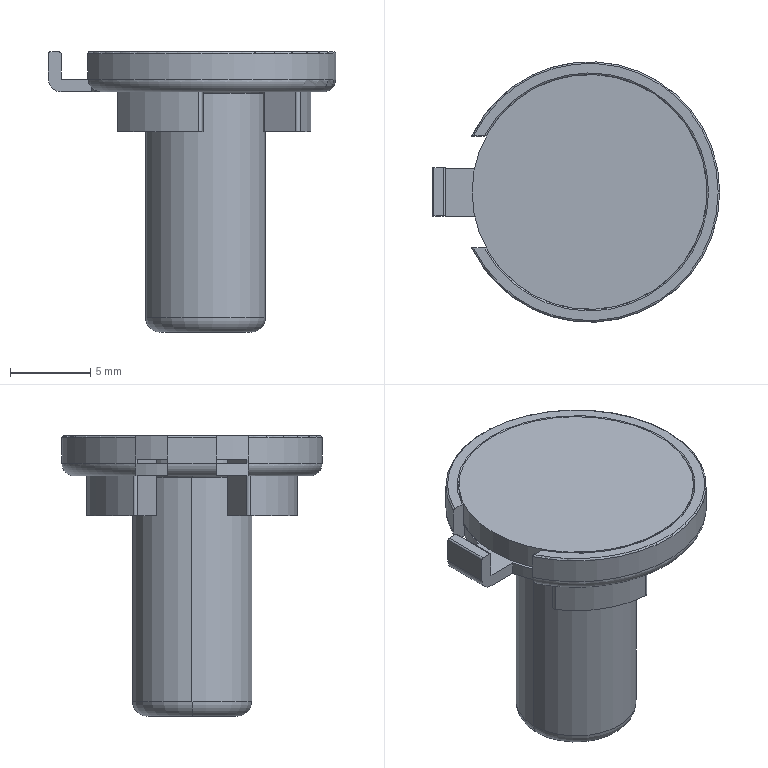NC program | NX | posted with a generic post | part box 17.958 x 16.273 x 17.5 mm
Lines 901 to 1957 of 9718:
(ZLEVEL_PROFILE_COPY_1 , TOOL : D2)
N1782 T02 M6
N1784 G54
N1786 G17 G0 G90 X-10.478 Y2.889 S6500 M3
N1788 G43 Z10.5 H2
N1790 Z-0.04
N1792 G94 G1 X-10.31 Y2.598 F1250.
N1794 G3 X-10.137 Y2.498 R0.2
N1796 G1 X-9.965
N1798 X-9.951 Y2.5
N1800 X-8.536
N1802 G3 X-8.362 Y2.6 R0.2
N1804 G1 X-9.107 Y2.9
N1806 G0 X-10.478 Y2.889 Z-0.079
N1808 G1 X-10.31 Y2.598
N1810 G3 X-10.137 Y2.498 R0.2
N1812 G1 X-9.965
N1814 X-9.951 Y2.5
N1816 X-8.536
N1818 G3 X-8.362 Y2.6 R0.2
N1820 G1 X-9.108 Y2.9
N1822 G0 X-10.478 Y2.889 Z-0.119
N1824 G1 X-10.31 Y2.598
N1826 G3 X-10.137 Y2.498 R0.2
N1828 G1 X-10.04
N1830 X-9.976 Y2.488
N1832 X-9.965 Y2.498
N1834 X-9.801 Y2.5
N1836 X-8.536
N1838 G3 X-8.362 Y2.6 R0.2
N1840 G1 X-9.108 Y2.9
N1842 G0 X-10.479 Y2.889 Z-0.159
N1844 G1 X-10.31 Y2.598
N1846 G3 X-10.137 Y2.498 R0.2
N1848 G1 X-10.04
N1850 X-9.976 Y2.488
N1852 X-9.965 Y2.498
N1854 X-9.801 Y2.5
N1856 X-8.536
N1858 G3 X-8.362 Y2.6 R0.2
N1860 G1 X-9.108 Y2.9
N1862 G0 X-10.479 Y2.889 Z-0.198
N1864 G1 X-10.311 Y2.598
N1866 G3 X-10.137 Y2.498 R0.2
N1868 G1 X-10.04
N1870 X-9.976 Y2.488
N1872 X-9.965 Y2.498
N1874 X-9.801 Y2.5
N1876 X-8.536
N1878 G3 X-8.362 Y2.6 R0.2
N1880 G1 X-9.108 Y2.9
N1882 G0 X-10.479 Y2.889 Z-0.238
N1884 G1 X-10.311 Y2.598
N1886 G3 X-10.138 Y2.498 R0.2
N1888 G1 X-10.04
N1890 X-9.976 Y2.488
N1892 X-9.965 Y2.498
N1894 X-9.801 Y2.5
N1896 X-8.536
N1898 G3 X-8.362 Y2.6 R0.2
N1900 G1 X-9.108 Y2.9
N1902 G0 X-10.479 Y2.889 Z-0.278
N1904 G1 X-10.311 Y2.598
N1906 G3 X-10.138 Y2.498 R0.2
N1908 G1 X-10.04
N1910 X-9.976 Y2.488
N1912 X-9.965 Y2.498
N1914 X-9.801 Y2.5
N1916 X-8.536
N1918 G3 X-8.362 Y2.6 R0.2
N1920 G1 X-9.108 Y2.9
N1922 G0 X-10.479 Y2.889 Z-0.317
N1924 G1 X-10.311 Y2.598
N1926 G3 X-10.138 Y2.498 R0.2
N1928 G1 X-10.04
N1930 X-9.976 Y2.488
N1932 X-9.965 Y2.498
N1934 X-9.801 Y2.5
N1936 X-8.536
N1938 G3 X-8.362 Y2.6 R0.2
N1940 G1 X-9.108 Y2.9
N1942 G0 X-10.479 Y2.889 Z-0.357
N1944 G1 X-10.311 Y2.598
N1946 G3 X-10.138 Y2.498 R0.2
N1948 G1 X-10.04
N1950 X-9.976 Y2.488
N1952 X-9.965 Y2.498
N1954 X-9.801 Y2.5
N1956 X-8.536
N1958 G3 X-8.362 Y2.6 R0.2
N1960 G1 X-9.108 Y2.9
N1962 G0 X-10.479 Y2.889 Z-0.397
N1964 G1 X-10.311 Y2.598
N1966 G3 X-10.138 Y2.498 R0.2
N1968 G1 X-10.04
N1970 X-9.976 Y2.488
N1972 X-9.965 Y2.498
N1974 X-9.801 Y2.5
N1976 X-8.536
N1978 G3 X-8.362 Y2.6 R0.2
N1980 G1 X-9.108 Y2.9
N1982 G0 X-10.479 Y2.889 Z-0.437
N1984 G1 X-10.311 Y2.598
N1986 G3 X-10.138 Y2.498 R0.2
N1988 G1 X-10.04
N1990 X-9.976 Y2.488
N1992 X-9.965 Y2.498
N1994 X-9.801 Y2.5
N1996 X-8.536
N1998 G3 X-8.362 Y2.6 R0.2
N2000 G1 X-9.108 Y2.9
N2002 G0 X-10.48 Y2.889 Z-0.476
N2004 G1 X-10.312 Y2.598
N2006 G3 X-10.138 Y2.498 R0.2
N2008 G1 X-10.04
N2010 X-9.976 Y2.488
N2012 X-9.965 Y2.498
N2014 X-9.801 Y2.5
N2016 X-8.536
N2018 G3 X-8.362 Y2.6 R0.2
N2020 G1 X-9.108 Y2.9
N2022 G0 X-10.48 Y2.889 Z-0.516
N2024 G1 X-10.312 Y2.598
N2026 G3 X-10.139 Y2.498 R0.2
N2028 G1 X-10.04
N2030 X-9.976 Y2.488
N2032 X-9.965 Y2.498
N2034 X-9.801 Y2.5
N2036 X-8.536
N2038 G3 X-8.362 Y2.6 R0.2
N2040 G1 X-9.108 Y2.9
N2042 G0 X-10.48 Y2.889 Z-0.556
N2044 G1 X-10.312 Y2.598
N2046 G3 X-10.139 Y2.498 R0.2
N2048 G1 X-10.04
N2050 X-9.976 Y2.488
N2052 X-9.965 Y2.498
N2054 X-9.801 Y2.5
N2056 X-8.536
N2058 G3 X-8.362 Y2.6 R0.2
N2060 G1 X-9.108 Y2.9
N2062 G0 X-10.48 Y2.889 Z-0.595
N2064 G1 X-10.312 Y2.598
N2066 G3 X-10.139 Y2.498 R0.2
N2068 G1 X-10.04
N2070 X-9.976 Y2.488
N2072 X-9.965 Y2.498
N2074 X-9.801 Y2.5
N2076 X-8.536
N2078 G3 X-8.362 Y2.6 R0.2
N2080 G1 X-9.108 Y2.9
N2082 G0 X-10.48 Y2.889 Z-0.635
N2084 G1 X-10.312 Y2.598
N2086 G3 X-10.139 Y2.498 R0.2
N2088 G1 X-10.04
N2090 X-9.976 Y2.488
N2092 X-9.965 Y2.498
N2094 X-9.801 Y2.5
N2096 X-8.536
N2098 G3 X-8.362 Y2.6 R0.2
N2100 G1 X-9.108 Y2.9
N2102 G0 X-10.48 Y2.889 Z-0.675
N2104 G1 X-10.312 Y2.598
N2106 G3 X-10.139 Y2.498 R0.2
N2108 G1 X-10.04
N2110 X-9.976 Y2.488
N2112 X-9.965 Y2.498
N2114 X-9.801 Y2.5
N2116 X-8.536
N2118 G3 X-8.362 Y2.6 R0.2
N2120 G1 X-9.108 Y2.9
N2122 G0 X-10.48 Y2.889 Z-0.714
N2124 G1 X-10.313 Y2.599
N2126 G3 X-10.139 Y2.498 R0.2
N2128 G1 X-10.04
N2130 X-9.976 Y2.488
N2132 X-9.965 Y2.498
N2134 X-9.801 Y2.5
N2136 X-8.536
N2138 G3 X-8.362 Y2.6 R0.2
N2140 G1 X-9.108 Y2.9
N2142 G0 X-10.48 Y2.889 Z-0.754
N2144 G1 X-10.313 Y2.599
N2146 G3 X-10.14 Y2.498 R0.2
N2148 G1 X-10.04
N2150 X-9.976 Y2.488
N2152 X-9.965 Y2.498
N2154 X-9.801 Y2.5
N2156 X-8.536
N2158 G3 X-8.362 Y2.6 R0.2
N2160 G1 X-9.108 Y2.9
N2162 G0 X-10.48 Y2.889 Z-0.794
N2164 G1 X-10.313 Y2.599
N2166 G3 X-10.14 Y2.499 R0.2
N2168 G1 X-10.04 Y2.498
N2170 X-9.976 Y2.488
N2172 X-9.965 Y2.498
N2174 X-9.801 Y2.5
N2176 X-8.536
N2178 G3 X-8.362 Y2.6 R0.2
N2180 G1 X-9.108 Y2.9
N2182 G0 X-10.481 Y2.889 Z-0.833
N2184 G1 X-10.313 Y2.599
N2186 G3 X-10.14 Y2.499 R0.2
N2188 G1 X-10.04 Y2.498
N2190 X-9.976 Y2.488
N2192 X-9.965 Y2.498
N2194 X-9.801 Y2.5
N2196 X-8.536
N2198 G3 X-8.362 Y2.6 R0.2
N2200 G1 X-9.108 Y2.9
N2202 G0 X-10.481 Y2.89 Z-0.873
N2204 G1 X-10.313 Y2.599
N2206 G3 X-10.14 Y2.499 R0.2
N2208 G1 X-10.04 Y2.498
N2210 X-9.976 Y2.488
N2212 X-9.965 Y2.498
N2214 X-9.801 Y2.5
N2216 X-8.536
N2218 G3 X-8.362 Y2.6 R0.2
N2220 G1 X-9.108 Y2.9
N2222 G0 X-10.481 Y2.89 Z-0.913
N2224 G1 X-10.313 Y2.599
N2226 G3 X-10.14 Y2.499 R0.2
N2228 G1 X-10.04
N2230 X-9.976 Y2.488
N2232 X-9.965 Y2.499
N2234 X-9.801 Y2.5
N2236 X-8.536
N2238 G3 X-8.362 Y2.6 R0.2
N2240 G1 X-9.108 Y2.9
N2242 G0 X-10.481 Y2.89 Z-0.952
N2244 G1 X-10.313 Y2.599
N2246 G3 X-10.14 Y2.499 R0.2
N2248 G1 X-10.04
N2250 X-9.976 Y2.488
N2252 X-9.965 Y2.499
N2254 X-9.801 Y2.5
N2256 X-8.536
N2258 G3 X-8.362 Y2.6 R0.2
N2260 G1 X-9.108 Y2.9
N2262 G0 X-10.481 Y2.89 Z-0.992
N2264 G1 X-10.314 Y2.599
N2266 G3 X-10.14 Y2.499 R0.2
N2268 G1 X-10.04
N2270 X-9.976 Y2.488
N2272 X-9.965 Y2.499
N2274 X-9.801 Y2.5
N2276 X-8.536
N2278 G3 X-8.362 Y2.6 R0.2
N2280 G1 X-9.108 Y2.9
N2282 G0 X-10.481 Y2.89 Z-1.032
N2284 G1 X-10.314 Y2.599
N2286 G3 X-10.141 Y2.499 R0.2
N2288 G1 X-10.04
N2290 X-9.976 Y2.488
N2292 X-9.965 Y2.499
N2294 X-9.801 Y2.5
N2296 X-8.536
N2298 G3 X-8.362 Y2.6 R0.2
N2300 G1 X-9.108 Y2.9
N2302 G0 X-10.481 Y2.89 Z-1.071
N2304 G1 X-10.314 Y2.599
N2306 G3 X-10.141 Y2.499 R0.2
N2308 G1 X-10.04
N2310 X-9.976 Y2.488
N2312 X-9.965 Y2.499
N2314 X-9.801 Y2.5
N2316 X-8.536
N2318 G3 X-8.362 Y2.6 R0.2
N2320 G1 X-9.108 Y2.9
N2322 G0 X-10.481 Y2.89 Z-1.111
N2324 G1 X-10.314 Y2.599
N2326 G3 X-10.141 Y2.499 R0.2
N2328 G1 X-10.04
N2330 X-9.976 Y2.488
N2332 X-9.965 Y2.499
N2334 X-9.801 Y2.5
N2336 X-8.536
N2338 G3 X-8.362 Y2.6 R0.2
N2340 G1 X-9.108 Y2.9
N2342 G0 X-10.481 Y2.89 Z-1.151
N2344 G1 X-10.314 Y2.599
N2346 G3 X-10.141 Y2.499 R0.2
N2348 G1 X-10.04
N2350 X-9.976 Y2.488
N2352 X-9.965 Y2.499
N2354 X-9.801 Y2.5
N2356 X-8.536
N2358 G3 X-8.362 Y2.6 R0.2
N2360 G1 X-9.108 Y2.9
N2362 G0 X-10.482 Y2.89 Z-1.19
N2364 G1 X-10.314 Y2.599
N2366 G3 X-10.141 Y2.499 R0.2
N2368 G1 X-10.04
N2370 X-9.976 Y2.488
N2372 X-9.965 Y2.499
N2374 X-9.801 Y2.5
N2376 X-8.536
N2378 G3 X-8.362 Y2.6 R0.2
N2380 G1 X-9.109 Y2.9
N2382 G0 X-10.482 Y2.89 Z-1.23
N2384 G1 X-10.314 Y2.599
N2386 G3 X-10.141 Y2.499 R0.2
N2388 G1 X-10.04
N2390 X-9.976 Y2.488
N2392 X-9.965 Y2.499
N2394 X-9.801 Y2.5
N2396 X-7.882
N2398 G0 X-10.482 Y2.89 Z-1.27
N2400 G1 X-10.315 Y2.599
N2402 G3 X-10.142 Y2.499 R0.2
N2404 G1 X-10.04
N2406 X-9.976 Y2.488
N2408 X-9.965 Y2.499
N2410 X-9.801 Y2.5
N2412 X-7.882
N2414 G0 X-10.482 Y2.89 Z-1.31
N2416 G1 X-10.315 Y2.599
N2418 G3 X-10.142 Y2.499 R0.2
N2420 G1 X-10.04
N2422 X-9.976 Y2.488
N2424 X-9.965 Y2.499
N2426 X-9.801 Y2.5
N2428 X-7.883
N2430 G0 X-10.482 Y2.89 Z-1.349
N2432 G1 X-10.315 Y2.599
N2434 G3 X-10.142 Y2.499 R0.2
N2436 G1 X-10.04
N2438 X-9.976 Y2.488
N2440 X-9.965 Y2.499
N2442 X-9.801 Y2.5
N2444 X-7.883
N2446 G0 X-10.482 Y2.89 Z-1.389
N2448 G1 X-10.315 Y2.599
N2450 G3 X-10.142 Y2.499 R0.2
N2452 G1 X-10.04
N2454 X-9.976 Y2.488
N2456 X-9.965 Y2.499
N2458 X-9.801 Y2.5
N2460 X-7.883
N2462 G0 X-10.482 Y2.89 Z-1.429
N2464 G1 X-10.315 Y2.6
N2466 G3 X-10.142 Y2.499 R0.2
N2468 G1 X-10.04
N2470 X-9.976 Y2.488
N2472 X-9.965 Y2.499
N2474 X-9.801 Y2.5
N2476 X-7.884
N2478 G0 X-10.482 Y2.89 Z-1.468
N2480 G1 X-10.315 Y2.6
N2482 G3 X-10.142 Y2.499 R0.2
N2484 G1 X-10.04
N2486 X-9.976 Y2.488
N2488 X-9.965 Y2.499
N2490 X-9.801 Y2.5
N2492 X-7.884
N2494 G0 X-10.482 Y2.89 Z-1.508
N2496 G1 X-10.316 Y2.6
N2498 G3 X-10.142 Y2.499 R0.2
N2500 G1 X-10.04
N2502 X-9.976 Y2.488
N2504 X-9.965 Y2.499
N2506 X-9.801 Y2.5
N2508 X-7.884
N2510 G0 X-10.483 Y2.89 Z-1.548
N2512 G1 X-10.316 Y2.6
N2514 G3 X-10.143 Y2.499 R0.2
N2516 G1 X-10.04
N2518 X-9.976 Y2.488
N2520 X-9.965 Y2.499
N2522 X-9.801 Y2.5
N2524 X-7.885
N2526 G0 X-10.483 Y2.89 Z-1.587
N2528 G1 X-10.316 Y2.6
N2530 G3 X-10.143 Y2.499 R0.2
N2532 G1 X-10.04
N2534 X-9.976 Y2.488
N2536 X-9.965 Y2.499
N2538 X-9.801 Y2.5
N2540 X-7.885
N2542 G0 X-10.483 Y2.89 Z-1.627
N2544 G1 X-10.316 Y2.6
N2546 G3 X-10.143 Y2.499 R0.2
N2548 G1 X-10.04
N2550 X-9.976 Y2.488
N2552 X-9.965 Y2.499
N2554 X-9.801 Y2.5
N2556 X-7.885
N2558 G0 X-10.483 Y2.89 Z-1.667
N2560 G1 X-10.316 Y2.6
N2562 G3 X-10.143 Y2.499 R0.2
N2564 G1 X-10.04
N2566 X-9.976 Y2.488
N2568 X-9.965 Y2.499
N2570 X-9.801 Y2.5
N2572 X-7.886
N2574 G0 X-10.483 Y2.89 Z-1.706
N2576 G1 X-10.316 Y2.6
N2578 G3 X-10.143 Y2.5 R0.2
N2580 G1 X-10.04 Y2.499
N2582 X-9.976 Y2.488
N2584 X-9.965 Y2.499
N2586 X-9.801 Y2.5
N2588 X-7.886
N2590 G0 X-10.483 Y2.89 Z-1.746
N2592 G1 X-10.316 Y2.6
N2594 G3 X-10.143 Y2.5 R0.2
N2596 G1 X-10.04 Y2.499
N2598 X-9.976 Y2.488
N2600 X-9.965 Y2.499
N2602 X-9.801 Y2.5
N2604 X-7.886
N2606 G0 X-10.483 Y2.89 Z-1.786
N2608 G1 X-10.317 Y2.6
N2610 G3 X-10.144 Y2.5 R0.2
N2612 G1 X-10.04 Y2.499
N2614 X-9.976 Y2.488
N2616 X-9.965 Y2.499
N2618 X-9.801 Y2.5
N2620 X-7.886
N2622 G0 X-10.484 Y2.89 Z-1.825
N2624 G1 X-10.317 Y2.6
N2626 G3 X-10.144 Y2.5 R0.2
N2628 G1 X-10.04 Y2.499
N2630 X-9.976 Y2.488
N2632 X-9.965 Y2.499
N2634 X-9.801 Y2.5
N2636 X-7.886
N2638 G0 X-10.484 Y2.89 Z-1.865
N2640 G1 X-10.317 Y2.6
N2642 G3 X-10.144 Y2.5 R0.2
N2644 G1 X-10.04 Y2.499
N2646 X-9.976 Y2.488
N2648 X-9.965 Y2.499
N2650 X-9.801 Y2.5
N2652 X-7.886
N2654 G0 X-10.484 Y2.89 Z-1.905
N2656 G1 X-10.317 Y2.6
N2658 G3 X-10.144 Y2.5 R0.2
N2660 G1 X-10.04 Y2.499
N2662 X-9.976 Y2.488
N2664 X-9.965 Y2.499
N2666 X-9.795 Y2.5
N2668 X-7.886
N2670 G0 X-10.484 Y2.89 Z-1.944
N2672 G1 X-10.317 Y2.6
N2674 G3 X-10.144 Y2.5 R0.2
N2676 G1 X-10.04 Y2.499
N2678 X-9.976 Y2.488
N2680 X-9.965 Y2.499
N2682 X-9.785 Y2.5
N2684 X-7.886
N2686 G0 X-10.484 Y2.89 Z-1.984
N2688 G1 X-10.317 Y2.6
N2690 G3 X-10.144 Y2.5 R0.2
N2692 G1 X-10.04
N2694 X-9.976 Y2.488
N2696 X-9.965 Y2.499
N2698 X-9.785 Y2.5
N2700 X-7.886
N2702 G0 X-10.485 Y2.89 Z-2.024
N2704 G1 X-10.318 Y2.6
N2706 G3 X-10.145 Y2.5 R0.2
N2708 G1 X-10.04
N2710 X-9.976 Y2.488
N2712 X-9.965 Y2.5
N2714 X-9.785
N2716 X-7.886
N2718 G0 X-10.485 Y2.89 Z-2.063
N2720 G1 X-10.318 Y2.6
N2722 G3 X-10.145 Y2.5 R0.2
N2724 G1 X-10.04
N2726 X-9.976 Y2.488
N2728 X-9.965 Y2.5
N2730 X-9.785
N2732 X-7.886
N2734 G0 X-10.485 Y2.89 Z-2.103
N2736 G1 X-10.318 Y2.6
N2738 G3 X-10.145 Y2.5 R0.2
N2740 G1 X-10.04
N2742 X-9.976 Y2.488
N2744 X-9.965 Y2.5
N2746 X-9.785
N2748 X-7.886
N2750 G0 X-10.485 Y2.89 Z-2.143
N2752 G1 X-10.318 Y2.6
N2754 G3 X-10.145 Y2.5 R0.2
N2756 G1 X-10.04
N2758 X-9.976 Y2.488
N2760 X-9.965 Y2.5
N2762 X-9.785
N2764 X-7.886
N2766 G0 X-10.485 Y2.89 Z-2.183
N2768 G1 X-10.318 Y2.6
N2770 G3 X-10.145 Y2.5 R0.2
N2772 G1 X-10.04
N2774 X-9.976 Y2.488
N2776 X-9.965 Y2.5
N2778 X-9.785
N2780 X-7.886
N2782 G0 X-10.486 Y2.89 Z-2.222
N2784 G1 X-10.318 Y2.6
N2786 G3 X-10.145 Y2.5 R0.2
N2788 G1 X-10.04
N2790 X-9.976 Y2.488
N2792 X-9.965 Y2.5
N2794 X-9.785
N2796 X-7.886
N2798 G0 X-10.486 Y2.89 Z-2.262
N2800 G1 X-10.319 Y2.6
N2802 G3 X-10.145 Y2.5 R0.2
N2804 G1 X-10.04
N2806 X-9.976 Y2.488
N2808 X-9.965 Y2.5
N2810 X-9.785
N2812 X-7.886
N2814 G0 X-10.486 Y2.89 Z-2.302
N2816 G1 X-10.319 Y2.6
N2818 G3 X-10.146 Y2.5 R0.2
N2820 G1 X-10.04
N2822 X-9.976 Y2.488
N2824 X-9.965 Y2.5
N2826 X-9.785
N2828 X-7.886
N2830 G0 X-10.486 Y2.89 Z-2.341
N2832 G1 X-10.319 Y2.6
N2834 G3 X-10.146 Y2.5 R0.2
N2836 G1 X-10.04
N2838 X-9.976 Y2.488
N2840 X-9.965 Y2.5
N2842 X-9.785
N2844 X-7.886
N2846 G0 X-10.486 Y2.89 Z-2.381
N2848 G1 X-10.319 Y2.6
N2850 G3 X-10.146 Y2.5 R0.2
N2852 G1 X-10.04
N2854 X-9.976 Y2.488
N2856 X-9.965 Y2.5
N2858 X-9.785
N2860 X-7.886
N2862 G0 X-10.487 Y2.89 Z-2.421
N2864 G1 X-10.319 Y2.6
N2866 G3 X-10.146 Y2.5 R0.2
N2868 G1 X-10.04
N2870 X-9.976 Y2.488
N2872 X-9.965 Y2.5
N2874 X-9.785
N2876 X-7.886
N2878 G0 X-10.487 Y2.89 Z-2.46
N2880 G1 X-10.319 Y2.6
N2882 G3 X-10.146 Y2.5 R0.2
N2884 G1 X-10.04
N2886 X-9.976 Y2.488
N2888 X-9.965 Y2.5
N2890 X-9.785
N2892 X-7.886
N2894 G0 X-10.486 Y2.89 Z-2.5
N2896 G1 X-10.319 Y2.6
N2898 G3 X-10.146 Y2.5 R0.2
N2900 G1 X-10.027 Y2.499
N2902 X-9.976 Y2.488
N2904 X-9.965 Y2.5
N2906 X-9.785
N2908 X-7.886
N2910 G0 Z10.5
N2912 X-9.108 Y-2.9
N2914 Z-0.04
N2916 G1 X-8.356 Y-2.6
N2918 G3 X-8.529 Y-2.5 R0.2
N2920 G1 X-9.817
N2922 X-9.829 Y-2.497
N2924 X-10.135
N2926 G3 X-10.308 Y-2.597 R0.2
N2928 G1 X-10.477 Y-2.888
N2930 G0 X-9.109 Y-2.9 Z-0.079
N2932 G1 X-8.356 Y-2.6
N2934 G3 X-8.529 Y-2.5 R0.2
N2936 G1 X-9.82
N2938 X-10.135 Y-2.498
N2940 G3 X-10.309 Y-2.597 R0.2
N2942 G1 X-10.48 Y-2.888
N2944 G0 X-9.108 Y-2.9 Z-0.119
N2946 G1 X-8.356 Y-2.6
N2948 G3 X-8.529 Y-2.5 R0.2
N2950 G1 X-9.821
N2952 X-10.135 Y-2.498
N2954 G3 X-10.309 Y-2.597 R0.2
N2956 G1 X-10.48 Y-2.888
N2958 G0 X-9.108 Y-2.9 Z-0.159
N2960 G1 X-8.356 Y-2.6
N2962 G3 X-8.529 Y-2.5 R0.2
N2964 G1 X-9.821
N2966 X-10.135 Y-2.498
N2968 G3 X-10.309 Y-2.597 R0.2
N2970 G1 X-10.48 Y-2.888
N2972 G0 X-9.108 Y-2.9 Z-0.198
N2974 G1 X-8.356 Y-2.6
N2976 G3 X-8.529 Y-2.5 R0.2
N2978 G1 X-9.821
N2980 X-10.136 Y-2.498
N2982 G3 X-10.309 Y-2.597 R0.2
N2984 G1 X-10.48 Y-2.888
N2986 G0 X-9.108 Y-2.9 Z-0.238
N2988 G1 X-8.356 Y-2.6
N2990 G3 X-8.529 Y-2.5 R0.2
N2992 G1 X-9.821
N2994 X-10.136 Y-2.498
N2996 G3 X-10.309 Y-2.597 R0.2
N2998 G1 X-10.48 Y-2.888
N3000 G0 X-9.108 Y-2.9 Z-0.278
N3002 G1 X-8.356 Y-2.6
N3004 G3 X-8.529 Y-2.5 R0.2
N3006 G1 X-9.821
N3008 X-10.136 Y-2.498
N3010 G3 X-10.31 Y-2.597 R0.2
N3012 G1 X-10.48 Y-2.888
N3014 G0 X-9.109 Y-2.9 Z-0.317
N3016 G1 X-8.356 Y-2.6
N3018 G3 X-8.529 Y-2.5 R0.2
N3020 G1 X-9.821
N3022 X-10.136 Y-2.498
N3024 G3 X-10.31 Y-2.597 R0.2
N3026 G1 X-10.48 Y-2.888
N3028 G0 X-9.109 Y-2.9 Z-0.357
N3030 G1 X-8.356 Y-2.6
N3032 G3 X-8.529 Y-2.5 R0.2
N3034 G1 X-9.821
N3036 X-10.136 Y-2.498
N3038 G3 X-10.31 Y-2.597 R0.2
N3040 G1 X-10.48 Y-2.888
N3042 G0 X-9.109 Y-2.9 Z-0.397
N3044 G1 X-8.356 Y-2.6
N3046 G3 X-8.529 Y-2.5 R0.2
N3048 G1 X-9.821
N3050 X-10.136 Y-2.498
N3052 G3 X-10.31 Y-2.597 R0.2
N3054 G1 X-10.48 Y-2.888
N3056 G0 X-9.109 Y-2.9 Z-0.437
N3058 G1 X-8.356 Y-2.6
N3060 G3 X-8.529 Y-2.5 R0.2
N3062 G1 X-9.821
N3064 X-10.136 Y-2.498
N3066 G3 X-10.31 Y-2.597 R0.2
N3068 G1 X-10.48 Y-2.888
N3070 G0 X-9.109 Y-2.9 Z-0.476
N3072 G1 X-8.356 Y-2.6
N3074 G3 X-8.529 Y-2.5 R0.2
N3076 G1 X-9.821
N3078 X-10.136 Y-2.498
N3080 G3 X-10.31 Y-2.597 R0.2
N3082 G1 X-10.48 Y-2.888
N3084 G0 X-9.109 Y-2.9 Z-0.516
N3086 G1 X-8.356 Y-2.6
N3088 G3 X-8.529 Y-2.5 R0.2
N3090 G1 X-9.821
N3092 X-10.136 Y-2.498
N3094 G3 X-10.31 Y-2.597 R0.2
N3096 G1 X-10.48 Y-2.888
N3098 G0 X-9.109 Y-2.9 Z-0.556
N3100 G1 X-8.356 Y-2.6
N3102 G3 X-8.529 Y-2.5 R0.2
N3104 G1 X-9.821
N3106 X-10.136 Y-2.498
N3108 G3 X-10.31 Y-2.597 R0.2
N3110 G1 X-10.48 Y-2.888
N3112 G0 X-9.109 Y-2.9 Z-0.595
N3114 G1 X-8.356 Y-2.6
N3116 G3 X-8.529 Y-2.5 R0.2
N3118 G1 X-9.821
N3120 X-10.136 Y-2.498
N3122 G3 X-10.31 Y-2.597 R0.2
N3124 G1 X-10.48 Y-2.888
N3126 G0 X-9.109 Y-2.9 Z-0.635
N3128 G1 X-8.356 Y-2.6
N3130 G3 X-8.529 Y-2.5 R0.2
N3132 G1 X-9.821
N3134 X-10.136 Y-2.498
N3136 G3 X-10.31 Y-2.597 R0.2
N3138 G1 X-10.481 Y-2.888
N3140 G0 X-9.109 Y-2.9 Z-0.675
N3142 G1 X-8.356 Y-2.6
N3144 G3 X-8.529 Y-2.5 R0.2
N3146 G1 X-9.821
N3148 X-10.137 Y-2.498
N3150 G3 X-10.31 Y-2.597 R0.2
N3152 G1 X-10.481 Y-2.888
N3154 G0 X-9.109 Y-2.9 Z-0.714
N3156 G1 X-8.356 Y-2.6
N3158 G3 X-8.529 Y-2.5 R0.2
N3160 G1 X-9.821
N3162 X-10.137 Y-2.498
N3164 G3 X-10.31 Y-2.597 R0.2
N3166 G1 X-10.481 Y-2.888
N3168 G0 X-9.109 Y-2.9 Z-0.754
N3170 G1 X-8.356 Y-2.6
N3172 G3 X-8.529 Y-2.5 R0.2
N3174 G1 X-9.821
N3176 X-10.137 Y-2.498
N3178 G3 X-10.311 Y-2.597 R0.2
N3180 G1 X-10.481 Y-2.888
N3182 G0 X-9.109 Y-2.9 Z-0.794
N3184 G1 X-8.356 Y-2.6
N3186 G3 X-8.529 Y-2.5 R0.2
N3188 G1 X-9.821
N3190 X-10.137 Y-2.498
N3192 G3 X-10.311 Y-2.597 R0.2
N3194 G1 X-10.481 Y-2.888
N3196 G0 X-9.109 Y-2.9 Z-0.833
N3198 G1 X-8.356 Y-2.6
N3200 G3 X-8.529 Y-2.5 R0.2
N3202 G1 X-9.821
N3204 X-10.137 Y-2.498
N3206 G3 X-10.311 Y-2.597 R0.2
N3208 G1 X-10.481 Y-2.888
N3210 G0 X-9.109 Y-2.9 Z-0.873
N3212 G1 X-8.356 Y-2.6
N3214 G3 X-8.529 Y-2.5 R0.2
N3216 G1 X-9.821
N3218 X-10.137 Y-2.498
N3220 G3 X-10.311 Y-2.597 R0.2
N3222 G1 X-10.481 Y-2.888
N3224 G0 X-9.109 Y-2.9 Z-0.913
N3226 G1 X-8.356 Y-2.6
N3228 G3 X-8.529 Y-2.5 R0.2
N3230 G1 X-9.821
N3232 X-10.137 Y-2.498
N3234 G3 X-10.311 Y-2.597 R0.2
N3236 G1 X-10.481 Y-2.888
N3238 G0 X-9.109 Y-2.9 Z-0.952
N3240 G1 X-8.356 Y-2.6
N3242 G3 X-8.529 Y-2.5 R0.2
N3244 G1 X-9.821
N3246 X-10.137 Y-2.498
N3248 G3 X-10.311 Y-2.597 R0.2
N3250 G1 X-10.481 Y-2.888
N3252 G0 X-9.109 Y-2.9 Z-0.992
N3254 G1 X-8.356 Y-2.6
N3256 G3 X-8.529 Y-2.5 R0.2
N3258 G1 X-9.821
N3260 X-10.137 Y-2.498
N3262 G3 X-10.311 Y-2.597 R0.2
N3264 G1 X-10.481 Y-2.888
N3266 G0 X-9.109 Y-2.9 Z-1.032
N3268 G1 X-8.356 Y-2.6
N3270 G3 X-8.529 Y-2.5 R0.2
N3272 G1 X-9.821
N3274 X-10.137 Y-2.498
N3276 G3 X-10.311 Y-2.597 R0.2
N3278 G1 X-10.481 Y-2.888
N3280 G0 X-9.109 Y-2.9 Z-1.071
N3282 G1 X-8.356 Y-2.6
N3284 G3 X-8.529 Y-2.5 R0.2
N3286 G1 X-9.821
N3288 X-10.137 Y-2.498
N3290 G3 X-10.311 Y-2.597 R0.2
N3292 G1 X-10.481 Y-2.888
N3294 G0 X-9.109 Y-2.9 Z-1.111
N3296 G1 X-8.356 Y-2.6
N3298 G3 X-8.529 Y-2.5 R0.2
N3300 G1 X-9.821
N3302 X-10.138 Y-2.498
N3304 G3 X-10.311 Y-2.598 R0.2
N3306 G1 X-10.481 Y-2.888
N3308 G0 X-9.109 Y-2.9 Z-1.151
N3310 G1 X-8.356 Y-2.6
N3312 G3 X-8.529 Y-2.5 R0.2
N3314 G1 X-9.821
N3316 X-10.138 Y-2.498
N3318 G3 X-10.311 Y-2.598 R0.2
N3320 G1 X-10.481 Y-2.888
N3322 G0 X-9.109 Y-2.9 Z-1.19
N3324 G1 X-8.356 Y-2.6
N3326 G3 X-8.529 Y-2.5 R0.2
N3328 G1 X-9.821
N3330 X-10.138 Y-2.498
N3332 G3 X-10.311 Y-2.598 R0.2
N3334 G1 X-10.481 Y-2.888
N3336 G0 X-7.917 Y-2.503
N3338 G1 Z-1.23
N3340 X-7.927
N3342 X-7.884 Y-2.501
N3344 X-7.883 Y-2.497
N3346 X-7.911 Y-2.5
N3348 X-9.821
N3350 X-10.138 Y-2.498
N3352 G3 X-10.312 Y-2.598 R0.2
N3354 G1 X-10.481 Y-2.888
N3356 G0 X-7.918 Y-2.503
N3358 G1 Z-1.27
N3360 X-7.927
N3362 X-7.884 Y-2.501
N3364 X-7.883 Y-2.497
N3366 X-7.911 Y-2.5
N3368 X-9.821
N3370 X-10.138 Y-2.498
N3372 G3 X-10.312 Y-2.598 R0.2
N3374 G1 X-10.481 Y-2.888
N3376 G0 X-7.919 Y-2.503
N3378 G1 Z-1.31
N3380 X-7.927
N3382 X-7.884 Y-2.501
N3384 X-7.883 Y-2.497
N3386 X-7.911 Y-2.5
N3388 X-9.821
N3390 X-10.138 Y-2.498
N3392 G3 X-10.312 Y-2.598 R0.2
N3394 G1 X-10.481 Y-2.888
N3396 G0 X-7.92 Y-2.503
N3398 G1 Z-1.349
N3400 X-7.927
N3402 X-7.884 Y-2.501
N3404 X-7.883 Y-2.497
N3406 X-7.911 Y-2.5
N3408 X-9.821
N3410 X-10.138 Y-2.499
N3412 G3 X-10.312 Y-2.598 R0.2
N3414 G1 X-10.482 Y-2.889
N3416 G0 X-7.921 Y-2.503
N3418 G1 Z-1.389
N3420 X-7.884 Y-2.501
N3422 X-7.883 Y-2.497
N3424 X-7.911 Y-2.5
N3426 X-9.821
N3428 X-10.138 Y-2.499
N3430 G3 X-10.312 Y-2.598 R0.2
N3432 G1 X-10.482 Y-2.889
N3434 G0 X-7.922 Y-2.503
N3436 G1 Z-1.429
N3438 X-7.884 Y-2.501
N3440 X-7.883 Y-2.497
N3442 X-7.911 Y-2.5
N3444 X-9.821
N3446 X-10.138 Y-2.499
N3448 G3 X-10.312 Y-2.598 R0.2
N3450 G1 X-10.482 Y-2.889
N3452 G0 X-7.923 Y-2.503
N3454 G1 Z-1.468
N3456 X-7.884 Y-2.501
N3458 X-7.883 Y-2.497
N3460 X-7.911 Y-2.5
N3462 X-9.821
N3464 X-10.138 Y-2.499
N3466 G3 X-10.312 Y-2.598 R0.2
N3468 G1 X-10.482 Y-2.889
N3470 G0 X-7.924 Y-2.503
N3472 G1 Z-1.508
N3474 X-7.884 Y-2.501
N3476 X-7.883 Y-2.497
N3478 X-7.911 Y-2.5
N3480 X-9.821
N3482 X-10.138 Y-2.499
N3484 G3 X-10.312 Y-2.598 R0.2
N3486 G1 X-10.482 Y-2.889
N3488 G0 X-7.924 Y-2.503
N3490 G1 Z-1.548
N3492 X-7.884 Y-2.501
N3494 X-7.883 Y-2.497
N3496 X-7.911 Y-2.5
N3498 X-9.821
N3500 X-10.139 Y-2.499
N3502 G3 X-10.312 Y-2.598 R0.2
N3504 G1 X-10.482 Y-2.889
N3506 G0 X-7.925 Y-2.503
N3508 G1 Z-1.587
N3510 X-7.884 Y-2.501
N3512 X-7.883 Y-2.497
N3514 X-7.911 Y-2.5
N3516 X-9.821
N3518 X-10.139 Y-2.499
N3520 G3 X-10.312 Y-2.598 R0.2
N3522 G1 X-10.482 Y-2.889
N3524 G0 X-7.926 Y-2.503
N3526 G1 Z-1.627
N3528 X-7.928
N3530 X-7.884 Y-2.501
N3532 X-7.883 Y-2.497
N3534 X-7.911 Y-2.5
N3536 X-9.821
N3538 X-10.139 Y-2.499
N3540 G3 X-10.312 Y-2.598 R0.2
N3542 G1 X-10.482 Y-2.889
N3544 G0 X-7.929 Y-2.504
N3546 G1 Z-1.667
N3548 X-7.884 Y-2.501
N3550 X-7.883 Y-2.497
N3552 X-7.911 Y-2.5
N3554 X-9.821
N3556 X-10.139 Y-2.499
N3558 G3 X-10.312 Y-2.598 R0.2
N3560 G1 X-10.482 Y-2.889
N3562 G0 X-7.929 Y-2.504
N3564 G1 Z-1.706
N3566 X-7.884 Y-2.501
N3568 X-7.883 Y-2.497
N3570 X-7.911 Y-2.5
N3572 X-9.821
N3574 X-10.139 Y-2.499
N3576 G3 X-10.313 Y-2.598 R0.2
N3578 G1 X-10.482 Y-2.889
N3580 G0 X-7.929 Y-2.504
N3582 G1 Z-1.746
N3584 X-7.884 Y-2.501
N3586 X-7.883 Y-2.497
N3588 X-7.911 Y-2.5
N3590 X-9.819
N3592 X-9.829 Y-2.498
N3594 X-10.139
N3596 G3 X-10.312 Y-2.598 R0.2
N3598 G1 X-10.48 Y-2.889
N3600 G0 X-7.929 Y-2.504
N3602 G1 Z-1.786
N3604 X-7.884 Y-2.501
N3606 X-7.883 Y-2.497
N3608 X-7.911 Y-2.5
N3610 X-9.817
N3612 X-9.829 Y-2.498
N3614 X-10.139
N3616 G3 X-10.312 Y-2.598 R0.2
N3618 G1 X-10.48 Y-2.889
N3620 G0 X-7.929 Y-2.504
N3622 G1 Z-1.825
N3624 X-7.884 Y-2.501
N3626 X-7.883 Y-2.497
N3628 X-7.911 Y-2.5
N3630 X-9.817
N3632 X-9.829 Y-2.498
N3634 X-10.139
N3636 G3 X-10.312 Y-2.598 R0.2
N3638 G1 X-10.48 Y-2.889
N3640 G0 X-7.929 Y-2.504
N3642 G1 Z-1.865
N3644 X-7.884 Y-2.501
N3646 X-7.883 Y-2.497
N3648 X-7.911 Y-2.5
N3650 X-9.817
N3652 X-9.829 Y-2.498
N3654 X-10.139
N3656 G3 X-10.312 Y-2.598 R0.2
N3658 G1 X-10.48 Y-2.889
N3660 G0 X-7.929 Y-2.504
N3662 G1 Z-1.905
N3664 X-7.884 Y-2.501
N3666 X-7.883 Y-2.497
N3668 X-7.911 Y-2.5
N3670 X-9.817
N3672 X-9.829 Y-2.498
N3674 X-10.139
N3676 G3 X-10.313 Y-2.598 R0.2
N3678 G1 X-10.48 Y-2.889
N3680 G0 X-7.929 Y-2.504
N3682 G1 Z-1.944
N3684 X-7.884 Y-2.501
N3686 X-7.883 Y-2.497
N3688 X-7.911 Y-2.5
N3690 X-9.817
N3692 X-9.829 Y-2.498
N3694 X-10.139
N3696 G3 X-10.313 Y-2.598 R0.2
N3698 G1 X-10.48 Y-2.889
N3700 G0 X-7.929 Y-2.504
N3702 G1 Z-1.984
N3704 X-7.884 Y-2.501
N3706 X-7.883 Y-2.497
N3708 X-7.911 Y-2.5
N3710 X-9.817
N3712 X-9.829 Y-2.498
N3714 X-10.14
N3716 G3 X-10.313 Y-2.598 R0.2
N3718 G1 X-10.48 Y-2.889
N3720 G0 X-7.929 Y-2.504
N3722 G1 Z-2.024
N3724 X-7.884 Y-2.501
N3726 X-7.883 Y-2.497
N3728 X-7.911 Y-2.5
N3730 X-9.817
N3732 X-9.829 Y-2.498
N3734 X-10.14
N3736 G3 X-10.313 Y-2.598 R0.2
N3738 G1 X-10.48 Y-2.889
N3740 G0 X-7.929 Y-2.504
N3742 G1 Z-2.063
N3744 X-7.884 Y-2.501
N3746 X-7.883 Y-2.497
N3748 X-7.911 Y-2.5
N3750 X-9.817
N3752 X-9.829 Y-2.498
N3754 X-10.14
N3756 G3 X-10.313 Y-2.598 R0.2
N3758 G1 X-10.481 Y-2.889
N3760 G0 X-7.929 Y-2.504
N3762 G1 Z-2.103
N3764 X-7.884 Y-2.501
N3766 X-7.883 Y-2.497
N3768 X-7.911 Y-2.5
N3770 X-9.817
N3772 X-9.829 Y-2.498
N3774 X-10.14
N3776 G3 X-10.313 Y-2.598 R0.2
N3778 G1 X-10.481 Y-2.889
N3780 G0 X-7.929 Y-2.504
N3782 G1 Z-2.143
N3784 X-7.884 Y-2.501
N3786 X-7.883 Y-2.497
N3788 X-7.911 Y-2.5
N3790 X-9.817
N3792 X-9.829 Y-2.498
N3794 X-10.14
N3796 G3 X-10.313 Y-2.598 R0.2
N3798 G1 X-10.481 Y-2.889
N3800 G0 X-7.929 Y-2.504
N3802 G1 Z-2.183
N3804 X-7.884 Y-2.501
N3806 X-7.883 Y-2.497
N3808 X-7.911 Y-2.5
N3810 X-9.817
N3812 X-9.829 Y-2.498
N3814 X-10.14
N3816 G3 X-10.313 Y-2.598 R0.2
N3818 G1 X-10.481 Y-2.889
N3820 G0 X-7.929 Y-2.504
N3822 G1 Z-2.222
N3824 X-7.884 Y-2.501
N3826 X-7.883 Y-2.497
N3828 X-7.911 Y-2.5
N3830 X-9.817
N3832 X-9.829 Y-2.498
N3834 X-10.14
N3836 G3 X-10.313 Y-2.598 R0.2
N3838 G1 X-10.481 Y-2.889
N3840 G0 X-7.929 Y-2.504
N3842 G1 Z-2.262
N3844 X-7.884 Y-2.501
N3846 X-7.883 Y-2.497
N3848 X-7.911 Y-2.5
N3850 X-9.817
N3852 X-9.829 Y-2.498
N3854 X-10.14
N3856 G3 X-10.313 Y-2.598 R0.2
N3858 G1 X-10.481 Y-2.889
N3860 G0 X-7.929 Y-2.504
N3862 G1 Z-2.302
N3864 X-7.884 Y-2.501
N3866 X-7.883 Y-2.497
N3868 X-7.911 Y-2.5
N3870 X-9.817
N3872 X-9.829 Y-2.498
N3874 X-10.14
N3876 G3 X-10.313 Y-2.598 R0.2
N3878 G1 X-10.481 Y-2.889
N3880 G0 X-7.929 Y-2.504
N3882 G1 Z-2.341
N3884 X-7.884 Y-2.501
N3886 X-7.883 Y-2.497
N3888 X-7.911 Y-2.5